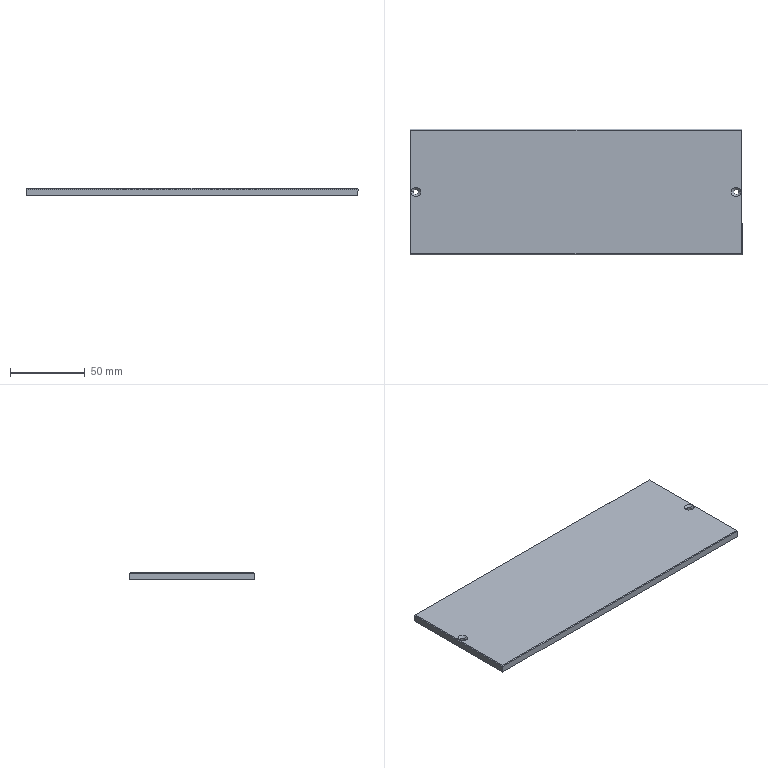Part | SolidWorks | features BaseBody 1 | 1 solid | 18 faces | box 222.8 x 84 x 5 mm | volume 93378 mm3 | plane 10 | cylinder 4 | cone 4 | commonest cylinder face diameters 3.4 x4
STEP:
#1=CARTESIAN_POINT('',(109.2,42.,1.));
#2=VERTEX_POINT('',#1);
#3=CARTESIAN_POINT('',(105.8,42.,1.));
#4=VERTEX_POINT('',#3);
#5=CARTESIAN_POINT('',(107.5,42.,1.));
#6=DIRECTION('',(0.,0.,-1.));
#7=DIRECTION('',(-1.,0.,0.));
#8=AXIS2_PLACEMENT_3D('',#5,#6,#7);
#9=CIRCLE('',#8,1.7);
#10=EDGE_CURVE('',#2,#4,#9,.T.);
#11=ORIENTED_EDGE('',*,*,#10,.F.);
#12=CARTESIAN_POINT('',(109.2,42.,-2.5));
#13=VERTEX_POINT('',#12);
#14=CARTESIAN_POINT('',(109.2,42.,2.5));
#15=DIRECTION('',(0.,0.,-1.));
#16=VECTOR('',#15,1000.);
#17=LINE('',#14,#16);
#18=EDGE_CURVE('',#2,#13,#17,.T.);
#19=ORIENTED_EDGE('',*,*,#18,.T.);
#20=CARTESIAN_POINT('',(105.8,42.,-2.5));
#21=VERTEX_POINT('',#20);
#22=CARTESIAN_POINT('',(107.5,42.,-2.5));
#23=DIRECTION('',(0.,0.,-1.));
#24=DIRECTION('',(-1.,0.,0.));
#25=AXIS2_PLACEMENT_3D('',#22,#23,#24);
#26=CIRCLE('',#25,1.7);
#27=EDGE_CURVE('',#13,#21,#26,.T.);
#28=ORIENTED_EDGE('',*,*,#27,.T.);
#29=CARTESIAN_POINT('',(105.8,42.,2.5));
#30=DIRECTION('',(0.,0.,-1.));
#31=VECTOR('',#30,1000.);
#32=LINE('',#29,#31);
#33=EDGE_CURVE('',#4,#21,#32,.T.);
#34=ORIENTED_EDGE('',*,*,#33,.F.);
#35=EDGE_LOOP('',(#11,#19,#28,#34));
#36=FACE_OUTER_BOUND('',#35,.T.);
#37=CARTESIAN_POINT('',(107.5,42.,2.5));
#38=DIRECTION('',(0.,0.,-1.));
#39=DIRECTION('',(-1.,0.,0.));
#40=AXIS2_PLACEMENT_3D('',#37,#38,#39);
#41=CYLINDRICAL_SURFACE('',#40,1.7);
#42=ADVANCED_FACE('',(#36),#41,.F.);
#43=CARTESIAN_POINT('',(-105.8,42.,1.));
#44=VERTEX_POINT('',#43);
#45=CARTESIAN_POINT('',(-109.2,42.,1.));
#46=VERTEX_POINT('',#45);
#47=CARTESIAN_POINT('',(-107.5,42.,1.));
#48=DIRECTION('',(0.,0.,-1.));
#49=DIRECTION('',(-1.,0.,0.));
#50=AXIS2_PLACEMENT_3D('',#47,#48,#49);
#51=CIRCLE('',#50,1.7);
#52=EDGE_CURVE('',#44,#46,#51,.T.);
#53=ORIENTED_EDGE('',*,*,#52,.F.);
#54=CARTESIAN_POINT('',(-105.8,42.,-2.5));
#55=VERTEX_POINT('',#54);
#56=CARTESIAN_POINT('',(-105.8,42.,2.5));
#57=DIRECTION('',(0.,0.,-1.));
#58=VECTOR('',#57,1000.);
#59=LINE('',#56,#58);
#60=EDGE_CURVE('',#44,#55,#59,.T.);
#61=ORIENTED_EDGE('',*,*,#60,.T.);
#62=CARTESIAN_POINT('',(-109.2,42.,-2.5));
#63=VERTEX_POINT('',#62);
#64=CARTESIAN_POINT('',(-107.5,42.,-2.5));
#65=DIRECTION('',(0.,0.,-1.));
#66=DIRECTION('',(-1.,0.,0.));
#67=AXIS2_PLACEMENT_3D('',#64,#65,#66);
#68=CIRCLE('',#67,1.7);
#69=EDGE_CURVE('',#55,#63,#68,.T.);
#70=ORIENTED_EDGE('',*,*,#69,.T.);
#71=CARTESIAN_POINT('',(-109.2,42.,2.5));
#72=DIRECTION('',(0.,0.,-1.));
#73=VECTOR('',#72,1000.);
#74=LINE('',#71,#73);
#75=EDGE_CURVE('',#46,#63,#74,.T.);
#76=ORIENTED_EDGE('',*,*,#75,.F.);
#77=EDGE_LOOP('',(#53,#61,#70,#76));
#78=FACE_OUTER_BOUND('',#77,.T.);
#79=CARTESIAN_POINT('',(-107.5,42.,2.5));
#80=DIRECTION('',(0.,0.,-1.));
#81=DIRECTION('',(-1.,0.,0.));
#82=AXIS2_PLACEMENT_3D('',#79,#80,#81);
#83=CYLINDRICAL_SURFACE('',#82,1.7);
#84=ADVANCED_FACE('',(#78),#83,.F.);
#85=ORIENTED_EDGE('',*,*,#10,.T.);
#86=CARTESIAN_POINT('',(104.3,42.,2.5));
#87=VERTEX_POINT('',#86);
#88=CARTESIAN_POINT('',(104.3,42.,2.5));
#89=DIRECTION('',(-0.7071,0.,0.7071));
#90=VECTOR('',#89,1000.);
#91=LINE('',#88,#90);
#92=EDGE_CURVE('',#4,#87,#91,.T.);
#93=ORIENTED_EDGE('',*,*,#92,.T.);
#94=CARTESIAN_POINT('',(110.7,42.,2.5));
#95=VERTEX_POINT('',#94);
#96=CARTESIAN_POINT('',(107.5,42.,2.5));
#97=DIRECTION('',(0.,0.,-1.));
#98=DIRECTION('',(1.,0.,0.));
#99=AXIS2_PLACEMENT_3D('',#96,#97,#98);
#100=CIRCLE('',#99,3.2);
#101=EDGE_CURVE('',#95,#87,#100,.T.);
#102=ORIENTED_EDGE('',*,*,#101,.F.);
#103=CARTESIAN_POINT('',(110.7,42.,2.5));
#104=DIRECTION('',(0.7071,0.,0.7071));
#105=VECTOR('',#104,1000.);
#106=LINE('',#103,#105);
#107=EDGE_CURVE('',#2,#95,#106,.T.);
#108=ORIENTED_EDGE('',*,*,#107,.F.);
#109=EDGE_LOOP('',(#85,#93,#102,#108));
#110=FACE_OUTER_BOUND('',#109,.T.);
#111=CARTESIAN_POINT('',(107.5,42.,2.5));
#112=DIRECTION('',(0.,0.,1.));
#113=DIRECTION('',(1.,0.,0.));
#114=AXIS2_PLACEMENT_3D('',#111,#112,#113);
#115=CONICAL_SURFACE('',#114,3.2,0.7854);
#116=ADVANCED_FACE('',(#110),#115,.F.);
#117=ORIENTED_EDGE('',*,*,#52,.T.);
#118=CARTESIAN_POINT('',(-110.7,42.,2.5));
#119=VERTEX_POINT('',#118);
#120=CARTESIAN_POINT('',(-110.7,42.,2.5));
#121=DIRECTION('',(-0.7071,0.,0.7071));
#122=VECTOR('',#121,1000.);
#123=LINE('',#120,#122);
#124=EDGE_CURVE('',#46,#119,#123,.T.);
#125=ORIENTED_EDGE('',*,*,#124,.T.);
#126=CARTESIAN_POINT('',(-104.3,42.,2.5));
#127=VERTEX_POINT('',#126);
#128=CARTESIAN_POINT('',(-107.5,42.,2.5));
#129=DIRECTION('',(0.,0.,-1.));
#130=DIRECTION('',(1.,0.,0.));
#131=AXIS2_PLACEMENT_3D('',#128,#129,#130);
#132=CIRCLE('',#131,3.2);
#133=EDGE_CURVE('',#127,#119,#132,.T.);
#134=ORIENTED_EDGE('',*,*,#133,.F.);
#135=CARTESIAN_POINT('',(-104.3,42.,2.5));
#136=DIRECTION('',(0.7071,0.,0.7071));
#137=VECTOR('',#136,1000.);
#138=LINE('',#135,#137);
#139=EDGE_CURVE('',#44,#127,#138,.T.);
#140=ORIENTED_EDGE('',*,*,#139,.F.);
#141=EDGE_LOOP('',(#117,#125,#134,#140));
#142=FACE_OUTER_BOUND('',#141,.T.);
#143=CARTESIAN_POINT('',(-107.5,42.,2.5));
#144=DIRECTION('',(0.,0.,1.));
#145=DIRECTION('',(1.,0.,0.));
#146=AXIS2_PLACEMENT_3D('',#143,#144,#145);
#147=CONICAL_SURFACE('',#146,3.2,0.7854);
#148=ADVANCED_FACE('',(#142),#147,.F.);
#149=CARTESIAN_POINT('',(107.5,42.,-2.5));
#150=DIRECTION('',(0.,0.,-1.));
#151=DIRECTION('',(-1.,0.,0.));
#152=AXIS2_PLACEMENT_3D('',#149,#150,#151);
#153=CIRCLE('',#152,1.7);
#154=EDGE_CURVE('',#21,#13,#153,.T.);
#155=ORIENTED_EDGE('',*,*,#154,.F.);
#156=ORIENTED_EDGE('',*,*,#27,.F.);
#157=EDGE_LOOP('',(#155,#156));
#158=FACE_BOUND('',#157,.T.);
#159=CARTESIAN_POINT('',(-107.5,42.,-2.5));
#160=DIRECTION('',(0.,0.,-1.));
#161=DIRECTION('',(-1.,0.,0.));
#162=AXIS2_PLACEMENT_3D('',#159,#160,#161);
#163=CIRCLE('',#162,1.7);
#164=EDGE_CURVE('',#63,#55,#163,.T.);
#165=ORIENTED_EDGE('',*,*,#164,.F.);
#166=ORIENTED_EDGE('',*,*,#69,.F.);
#167=EDGE_LOOP('',(#165,#166));
#168=FACE_BOUND('',#167,.T.);
#169=CARTESIAN_POINT('',(111.4,84.,-2.5));
#170=VERTEX_POINT('',#169);
#171=CARTESIAN_POINT('',(-111.4,84.,-2.5));
#172=VERTEX_POINT('',#171);
#173=CARTESIAN_POINT('',(0.,84.,-2.5));
#174=DIRECTION('',(-1.,0.,0.));
#175=VECTOR('',#174,1000.);
#176=LINE('',#173,#175);
#177=EDGE_CURVE('',#170,#172,#176,.T.);
#178=ORIENTED_EDGE('',*,*,#177,.F.);
#179=CARTESIAN_POINT('',(111.4,0.,-2.5));
#180=VERTEX_POINT('',#179);
#181=CARTESIAN_POINT('',(111.4,0.,-2.5));
#182=DIRECTION('',(0.,1.,0.));
#183=VECTOR('',#182,1000.);
#184=LINE('',#181,#183);
#185=EDGE_CURVE('',#180,#170,#184,.T.);
#186=ORIENTED_EDGE('',*,*,#185,.F.);
#187=CARTESIAN_POINT('',(-111.4,0.,-2.5));
#188=VERTEX_POINT('',#187);
#189=CARTESIAN_POINT('',(0.,0.,-2.5));
#190=DIRECTION('',(1.,0.,0.));
#191=VECTOR('',#190,1000.);
#192=LINE('',#189,#191);
#193=EDGE_CURVE('',#188,#180,#192,.T.);
#194=ORIENTED_EDGE('',*,*,#193,.F.);
#195=CARTESIAN_POINT('',(-111.4,0.,-2.5));
#196=DIRECTION('',(0.,-1.,0.));
#197=VECTOR('',#196,1000.);
#198=LINE('',#195,#197);
#199=EDGE_CURVE('',#172,#188,#198,.T.);
#200=ORIENTED_EDGE('',*,*,#199,.F.);
#201=EDGE_LOOP('',(#178,#186,#194,#200));
#202=FACE_OUTER_BOUND('',#201,.T.);
#203=CARTESIAN_POINT('',(0.,0.,-2.5));
#204=DIRECTION('',(0.,0.,1.));
#205=DIRECTION('',(1.,0.,0.));
#206=AXIS2_PLACEMENT_3D('',#203,#204,#205);
#207=PLANE('',#206);
#208=ADVANCED_FACE('',(#158,#168,#202),#207,.F.);
#209=ORIENTED_EDGE('',*,*,#18,.F.);
#210=CARTESIAN_POINT('',(107.5,42.,1.));
#211=DIRECTION('',(0.,0.,-1.));
#212=DIRECTION('',(-1.,0.,0.));
#213=AXIS2_PLACEMENT_3D('',#210,#211,#212);
#214=CIRCLE('',#213,1.7);
#215=EDGE_CURVE('',#4,#2,#214,.T.);
#216=ORIENTED_EDGE('',*,*,#215,.F.);
#217=ORIENTED_EDGE('',*,*,#33,.T.);
#218=ORIENTED_EDGE('',*,*,#154,.T.);
#219=EDGE_LOOP('',(#209,#216,#217,#218));
#220=FACE_OUTER_BOUND('',#219,.T.);
#221=CARTESIAN_POINT('',(107.5,42.,2.5));
#222=DIRECTION('',(0.,0.,-1.));
#223=DIRECTION('',(-1.,0.,0.));
#224=AXIS2_PLACEMENT_3D('',#221,#222,#223);
#225=CYLINDRICAL_SURFACE('',#224,1.7);
#226=ADVANCED_FACE('',(#220),#225,.F.);
#227=ORIENTED_EDGE('',*,*,#60,.F.);
#228=CARTESIAN_POINT('',(-107.5,42.,1.));
#229=DIRECTION('',(0.,0.,-1.));
#230=DIRECTION('',(-1.,0.,0.));
#231=AXIS2_PLACEMENT_3D('',#228,#229,#230);
#232=CIRCLE('',#231,1.7);
#233=EDGE_CURVE('',#46,#44,#232,.T.);
#234=ORIENTED_EDGE('',*,*,#233,.F.);
#235=ORIENTED_EDGE('',*,*,#75,.T.);
#236=ORIENTED_EDGE('',*,*,#164,.T.);
#237=EDGE_LOOP('',(#227,#234,#235,#236));
#238=FACE_OUTER_BOUND('',#237,.T.);
#239=CARTESIAN_POINT('',(-107.5,42.,2.5));
#240=DIRECTION('',(0.,0.,-1.));
#241=DIRECTION('',(-1.,0.,0.));
#242=AXIS2_PLACEMENT_3D('',#239,#240,#241);
#243=CYLINDRICAL_SURFACE('',#242,1.7);
#244=ADVANCED_FACE('',(#238),#243,.F.);
#245=CARTESIAN_POINT('',(-111.4,84.,2.));
#246=VERTEX_POINT('',#245);
#247=CARTESIAN_POINT('',(-111.4,0.,2.));
#248=VERTEX_POINT('',#247);
#249=CARTESIAN_POINT('',(-111.4,84.,2.));
#250=DIRECTION('',(0.,-1.,0.));
#251=VECTOR('',#250,1000.);
#252=LINE('',#249,#251);
#253=EDGE_CURVE('',#246,#248,#252,.T.);
#254=ORIENTED_EDGE('',*,*,#253,.F.);
#255=CARTESIAN_POINT('',(-111.4,84.,2.5));
#256=DIRECTION('',(0.,0.,1.));
#257=VECTOR('',#256,1000.);
#258=LINE('',#255,#257);
#259=EDGE_CURVE('',#172,#246,#258,.T.);
#260=ORIENTED_EDGE('',*,*,#259,.F.);
#261=ORIENTED_EDGE('',*,*,#199,.T.);
#262=CARTESIAN_POINT('',(-111.4,0.,2.5));
#263=DIRECTION('',(0.,0.,-1.));
#264=VECTOR('',#263,1000.);
#265=LINE('',#262,#264);
#266=EDGE_CURVE('',#248,#188,#265,.T.);
#267=ORIENTED_EDGE('',*,*,#266,.F.);
#268=EDGE_LOOP('',(#254,#260,#261,#267));
#269=FACE_OUTER_BOUND('',#268,.T.);
#270=CARTESIAN_POINT('',(-111.4,84.,2.5));
#271=DIRECTION('',(1.,0.,0.));
#272=DIRECTION('',(0.,0.,-1.));
#273=AXIS2_PLACEMENT_3D('',#270,#271,#272);
#274=PLANE('',#273);
#275=ADVANCED_FACE('',(#269),#274,.F.);
#276=CARTESIAN_POINT('',(111.4,84.,2.));
#277=VERTEX_POINT('',#276);
#278=CARTESIAN_POINT('',(-111.4,84.,2.));
#279=DIRECTION('',(-1.,0.,0.));
#280=VECTOR('',#279,1000.);
#281=LINE('',#278,#280);
#282=EDGE_CURVE('',#277,#246,#281,.T.);
#283=ORIENTED_EDGE('',*,*,#282,.F.);
#284=CARTESIAN_POINT('',(111.4,84.,2.5));
#285=DIRECTION('',(0.,0.,1.));
#286=VECTOR('',#285,1000.);
#287=LINE('',#284,#286);
#288=EDGE_CURVE('',#170,#277,#287,.T.);
#289=ORIENTED_EDGE('',*,*,#288,.F.);
#290=ORIENTED_EDGE('',*,*,#177,.T.);
#291=ORIENTED_EDGE('',*,*,#259,.T.);
#292=EDGE_LOOP('',(#283,#289,#290,#291));
#293=FACE_OUTER_BOUND('',#292,.T.);
#294=CARTESIAN_POINT('',(-111.4,84.,2.5));
#295=DIRECTION('',(0.,-1.,0.));
#296=DIRECTION('',(0.,0.,-1.));
#297=AXIS2_PLACEMENT_3D('',#294,#295,#296);
#298=PLANE('',#297);
#299=ADVANCED_FACE('',(#293),#298,.F.);
#300=CARTESIAN_POINT('',(111.4,0.,2.));
#301=VERTEX_POINT('',#300);
#302=CARTESIAN_POINT('',(111.4,0.,2.));
#303=DIRECTION('',(0.,1.,0.));
#304=VECTOR('',#303,1000.);
#305=LINE('',#302,#304);
#306=EDGE_CURVE('',#301,#277,#305,.T.);
#307=ORIENTED_EDGE('',*,*,#306,.F.);
#308=CARTESIAN_POINT('',(111.4,0.,2.5));
#309=DIRECTION('',(0.,0.,1.));
#310=VECTOR('',#309,1000.);
#311=LINE('',#308,#310);
#312=EDGE_CURVE('',#180,#301,#311,.T.);
#313=ORIENTED_EDGE('',*,*,#312,.F.);
#314=ORIENTED_EDGE('',*,*,#185,.T.);
#315=ORIENTED_EDGE('',*,*,#288,.T.);
#316=EDGE_LOOP('',(#307,#313,#314,#315));
#317=FACE_OUTER_BOUND('',#316,.T.);
#318=CARTESIAN_POINT('',(111.4,0.,2.5));
#319=DIRECTION('',(-1.,0.,0.));
#320=DIRECTION('',(0.,0.,1.));
#321=AXIS2_PLACEMENT_3D('',#318,#319,#320);
#322=PLANE('',#321);
#323=ADVANCED_FACE('',(#317),#322,.F.);
#324=CARTESIAN_POINT('',(-111.4,0.,2.));
#325=DIRECTION('',(1.,0.,0.));
#326=VECTOR('',#325,1000.);
#327=LINE('',#324,#326);
#328=EDGE_CURVE('',#248,#301,#327,.T.);
#329=ORIENTED_EDGE('',*,*,#328,.F.);
#330=ORIENTED_EDGE('',*,*,#266,.T.);
#331=ORIENTED_EDGE('',*,*,#193,.T.);
#332=ORIENTED_EDGE('',*,*,#312,.T.);
#333=EDGE_LOOP('',(#329,#330,#331,#332));
#334=FACE_OUTER_BOUND('',#333,.T.);
#335=CARTESIAN_POINT('',(-111.4,0.,2.5));
#336=DIRECTION('',(0.,1.,0.));
#337=DIRECTION('',(-1.,0.,0.));
#338=AXIS2_PLACEMENT_3D('',#335,#336,#337);
#339=PLANE('',#338);
#340=ADVANCED_FACE('',(#334),#339,.F.);
#341=ORIENTED_EDGE('',*,*,#92,.F.);
#342=ORIENTED_EDGE('',*,*,#215,.T.);
#343=ORIENTED_EDGE('',*,*,#107,.T.);
#344=CARTESIAN_POINT('',(107.5,42.,2.5));
#345=DIRECTION('',(0.,0.,-1.));
#346=DIRECTION('',(1.,0.,0.));
#347=AXIS2_PLACEMENT_3D('',#344,#345,#346);
#348=CIRCLE('',#347,3.2);
#349=EDGE_CURVE('',#87,#95,#348,.T.);
#350=ORIENTED_EDGE('',*,*,#349,.F.);
#351=EDGE_LOOP('',(#341,#342,#343,#350));
#352=FACE_OUTER_BOUND('',#351,.T.);
#353=CARTESIAN_POINT('',(107.5,42.,2.5));
#354=DIRECTION('',(0.,0.,1.));
#355=DIRECTION('',(1.,0.,0.));
#356=AXIS2_PLACEMENT_3D('',#353,#354,#355);
#357=CONICAL_SURFACE('',#356,3.2,0.7854);
#358=ADVANCED_FACE('',(#352),#357,.F.);
#359=ORIENTED_EDGE('',*,*,#124,.F.);
#360=ORIENTED_EDGE('',*,*,#233,.T.);
#361=ORIENTED_EDGE('',*,*,#139,.T.);
#362=CARTESIAN_POINT('',(-107.5,42.,2.5));
#363=DIRECTION('',(0.,0.,-1.));
#364=DIRECTION('',(1.,0.,0.));
#365=AXIS2_PLACEMENT_3D('',#362,#363,#364);
#366=CIRCLE('',#365,3.2);
#367=EDGE_CURVE('',#119,#127,#366,.T.);
#368=ORIENTED_EDGE('',*,*,#367,.F.);
#369=EDGE_LOOP('',(#359,#360,#361,#368));
#370=FACE_OUTER_BOUND('',#369,.T.);
#371=CARTESIAN_POINT('',(-107.5,42.,2.5));
#372=DIRECTION('',(0.,0.,1.));
#373=DIRECTION('',(1.,0.,0.));
#374=AXIS2_PLACEMENT_3D('',#371,#372,#373);
#375=CONICAL_SURFACE('',#374,3.2,0.7854);
#376=ADVANCED_FACE('',(#370),#375,.F.);
#377=CARTESIAN_POINT('',(-110.9,0.5,2.5));
#378=VERTEX_POINT('',#377);
#379=CARTESIAN_POINT('',(-111.4,0.,2.));
#380=DIRECTION('',(0.5774,0.5774,0.5774));
#381=VECTOR('',#380,1000.);
#382=LINE('',#379,#381);
#383=EDGE_CURVE('',#248,#378,#382,.T.);
#384=ORIENTED_EDGE('',*,*,#383,.T.);
#385=CARTESIAN_POINT('',(-110.9,83.5,2.5));
#386=VERTEX_POINT('',#385);
#387=CARTESIAN_POINT('',(-110.9,0.,2.5));
#388=DIRECTION('',(0.,1.,0.));
#389=VECTOR('',#388,1000.);
#390=LINE('',#387,#389);
#391=EDGE_CURVE('',#378,#386,#390,.T.);
#392=ORIENTED_EDGE('',*,*,#391,.T.);
#393=CARTESIAN_POINT('',(-110.9,83.5,2.5));
#394=DIRECTION('',(-0.5774,0.5774,-0.5774));
#395=VECTOR('',#394,1000.);
#396=LINE('',#393,#395);
#397=EDGE_CURVE('',#386,#246,#396,.T.);
#398=ORIENTED_EDGE('',*,*,#397,.T.);
#399=ORIENTED_EDGE('',*,*,#253,.T.);
#400=EDGE_LOOP('',(#384,#392,#398,#399));
#401=FACE_OUTER_BOUND('',#400,.T.);
#402=CARTESIAN_POINT('',(-110.9,0.,2.5));
#403=DIRECTION('',(-0.7071,0.,0.7071));
#404=DIRECTION('',(0.7071,0.,0.7071));
#405=AXIS2_PLACEMENT_3D('',#402,#403,#404);
#406=PLANE('',#405);
#407=ADVANCED_FACE('',(#401),#406,.T.);
#408=ORIENTED_EDGE('',*,*,#397,.F.);
#409=CARTESIAN_POINT('',(110.9,83.5,2.5));
#410=VERTEX_POINT('',#409);
#411=CARTESIAN_POINT('',(0.,83.5,2.5));
#412=DIRECTION('',(1.,0.,0.));
#413=VECTOR('',#412,1000.);
#414=LINE('',#411,#413);
#415=EDGE_CURVE('',#386,#410,#414,.T.);
#416=ORIENTED_EDGE('',*,*,#415,.T.);
#417=CARTESIAN_POINT('',(110.9,83.5,2.5));
#418=DIRECTION('',(0.5774,0.5774,-0.5774));
#419=VECTOR('',#418,1000.);
#420=LINE('',#417,#419);
#421=EDGE_CURVE('',#410,#277,#420,.T.);
#422=ORIENTED_EDGE('',*,*,#421,.T.);
#423=ORIENTED_EDGE('',*,*,#282,.T.);
#424=EDGE_LOOP('',(#408,#416,#422,#423));
#425=FACE_OUTER_BOUND('',#424,.T.);
#426=CARTESIAN_POINT('',(0.,83.5,2.5));
#427=DIRECTION('',(0.,0.7071,0.7071));
#428=DIRECTION('',(0.,-0.7071,0.7071));
#429=AXIS2_PLACEMENT_3D('',#426,#427,#428);
#430=PLANE('',#429);
#431=ADVANCED_FACE('',(#425),#430,.T.);
#432=ORIENTED_EDGE('',*,*,#421,.F.);
#433=CARTESIAN_POINT('',(110.9,0.5,2.5));
#434=VERTEX_POINT('',#433);
#435=CARTESIAN_POINT('',(110.9,0.,2.5));
#436=DIRECTION('',(0.,-1.,0.));
#437=VECTOR('',#436,1000.);
#438=LINE('',#435,#437);
#439=EDGE_CURVE('',#410,#434,#438,.T.);
#440=ORIENTED_EDGE('',*,*,#439,.T.);
#441=CARTESIAN_POINT('',(110.9,0.5,2.5));
#442=DIRECTION('',(0.5774,-0.5774,-0.5774));
#443=VECTOR('',#442,1000.);
#444=LINE('',#441,#443);
#445=EDGE_CURVE('',#434,#301,#444,.T.);
#446=ORIENTED_EDGE('',*,*,#445,.T.);
#447=ORIENTED_EDGE('',*,*,#306,.T.);
#448=EDGE_LOOP('',(#432,#440,#446,#447));
#449=FACE_OUTER_BOUND('',#448,.T.);
#450=CARTESIAN_POINT('',(110.9,0.,2.5));
#451=DIRECTION('',(0.7071,0.,0.7071));
#452=DIRECTION('',(0.7071,0.,-0.7071));
#453=AXIS2_PLACEMENT_3D('',#450,#451,#452);
#454=PLANE('',#453);
#455=ADVANCED_FACE('',(#449),#454,.T.);
#456=ORIENTED_EDGE('',*,*,#383,.F.);
#457=ORIENTED_EDGE('',*,*,#328,.T.);
#458=ORIENTED_EDGE('',*,*,#445,.F.);
#459=CARTESIAN_POINT('',(0.,0.5,2.5));
#460=DIRECTION('',(-1.,0.,0.));
#461=VECTOR('',#460,1000.);
#462=LINE('',#459,#461);
#463=EDGE_CURVE('',#434,#378,#462,.T.);
#464=ORIENTED_EDGE('',*,*,#463,.T.);
#465=EDGE_LOOP('',(#456,#457,#458,#464));
#466=FACE_OUTER_BOUND('',#465,.T.);
#467=CARTESIAN_POINT('',(0.,0.5,2.5));
#468=DIRECTION('',(0.,-0.7071,0.7071));
#469=DIRECTION('',(0.,-0.7071,-0.7071));
#470=AXIS2_PLACEMENT_3D('',#467,#468,#469);
#471=PLANE('',#470);
#472=ADVANCED_FACE('',(#466),#471,.T.);
#473=ORIENTED_EDGE('',*,*,#463,.F.);
#474=ORIENTED_EDGE('',*,*,#439,.F.);
#475=ORIENTED_EDGE('',*,*,#415,.F.);
#476=ORIENTED_EDGE('',*,*,#391,.F.);
#477=EDGE_LOOP('',(#473,#474,#475,#476));
#478=FACE_OUTER_BOUND('',#477,.T.);
#479=ORIENTED_EDGE('',*,*,#133,.T.);
#480=ORIENTED_EDGE('',*,*,#367,.T.);
#481=EDGE_LOOP('',(#479,#480));
#482=FACE_BOUND('',#481,.T.);
#483=ORIENTED_EDGE('',*,*,#101,.T.);
#484=ORIENTED_EDGE('',*,*,#349,.T.);
#485=EDGE_LOOP('',(#483,#484));
#486=FACE_BOUND('',#485,.T.);
#487=CARTESIAN_POINT('',(0.,0.,2.5));
#488=DIRECTION('',(0.,0.,1.));
#489=DIRECTION('',(1.,0.,0.));
#490=AXIS2_PLACEMENT_3D('',#487,#488,#489);
#491=PLANE('',#490);
#492=ADVANCED_FACE('',(#478,#482,#486),#491,.T.);
#493=CLOSED_SHELL('',(#42,#84,#116,#148,#208,#226,#244,#275,#299,#323,#340,#358,#376,#407,#431,#455,#472,#492));
#494=MANIFOLD_SOLID_BREP('',#493);
#495=CARTESIAN_POINT('',(0.,0.,0.));
#496=DIRECTION('',(0.,0.,1.));
#497=DIRECTION('',(1.,0.,0.));
#498=AXIS2_PLACEMENT_3D('',#495,#496,#497);
#499=(LENGTH_UNIT()NAMED_UNIT(*)SI_UNIT(.MILLI.,.METRE.));
#500=UNCERTAINTY_MEASURE_WITH_UNIT(LENGTH_MEASURE(0.00001),#499,'','');
#501=(NAMED_UNIT(*)PLANE_ANGLE_UNIT()SI_UNIT($,.RADIAN.));
#502=(NAMED_UNIT(*)SI_UNIT($,.STERADIAN.)SOLID_ANGLE_UNIT());
#503=(GEOMETRIC_REPRESENTATION_CONTEXT(3)GLOBAL_UNCERTAINTY_ASSIGNED_CONTEXT((#500))GLOBAL_UNIT_ASSIGNED_CONTEXT((#499,#501,#502))REPRESENTATION_CONTEXT('',''));
#504=ADVANCED_BREP_SHAPE_REPRESENTATION('',(#494,#498),#503);